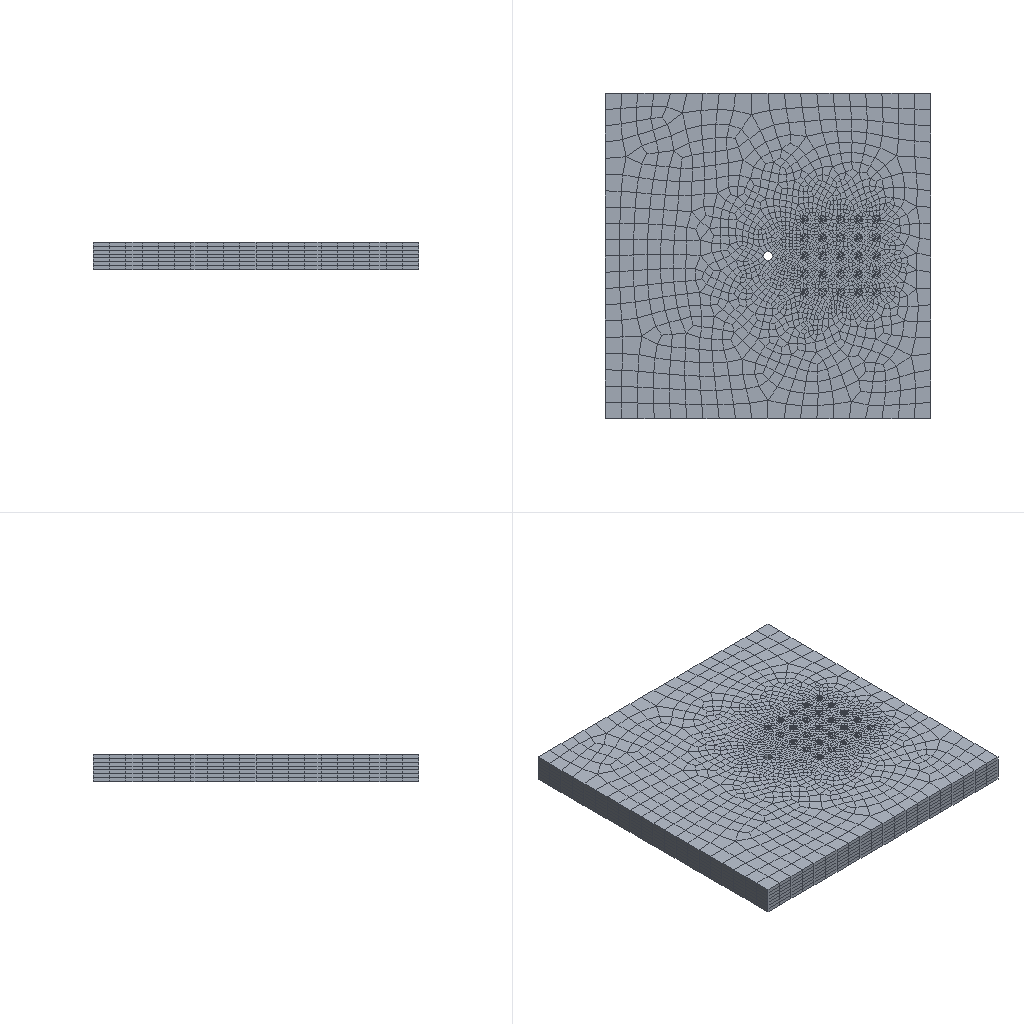Simulation study | abaqus
Set-up summary:
category,name,step,type,value,unit,region
solver,abaqus
solver,version,,,Abaqus/Standard 2020
units,not stated in the deck,,not stated
analysis,deck,,soils,soils
load_step,Step-1,Step-1,soils
load_step,requested,,,1
mesh,nodes,,,33552
mesh,elements,,,26299
element_type,C3D8R,,solid,13860
element_type,C3D8RP,,solid,12439
load,load commands in deck,,count,1
bc,support commands in deck,,count,5
material,SOIL,,in results
material,ZHUANG,,in results
check,setup vs results,,match,"per instance, exact: element labels, types and connectivity; labels of the nodes the elements use; coordinates of those nodes at SINGLE_PRECISION in 1 of 2 instance(s)"
Abaqus input file, long lists of numbers shortened:
*Heading
** Job name: Job-3 Model name: Model-1-Copy
** Generated by: Abaqus/CAE 2020
*Preprint, echo=NO, model=NO, history=NO, contact=NO
**
** PARTS
**
*Part, name=Part-1
*Node
      1,   17.1,           0.,           0.
      2,   15.3,           0.,           0.
** (15166 more lines like these left out)
*Element, type=C3D8RP
    1,   289,   327,   307,   328,  2185,  2223,  2203,  2224
    2,   327,   326,   306,   307,  2223,  2222,  2202,  2203
** (12437 more lines like these left out)
*Nset, nset=Set-1, generate
     1,  15168,      1
*Elset, elset=Set-1, generate
     1,  12439,      1
** Section: soil
*Solid Section, elset=Set-1, material=soil
,
*End Part
**
*Part, name=zhuang
*Node
      1,           3.,        -0.25,           0.
      2,           3.,        -0.25,          1.5
** (18382 more lines like these left out)
*Element, type=C3D8R
  1, 7899,  855,  870, 7901,  801,    1,   65,  803
  2, 7910, 7900,  857,  856,  812,  802,   52,   51
** (13858 more lines like these left out)
*Nset, nset=Set-1, generate
     1,  18384,      1
*Elset, elset=Set-1, generate
     1,  13860,      1
** Section: zhuang
*Solid Section, elset=Set-1, material=zhuang
,
*End Part
**
**
** ASSEMBLY
**
*Assembly, name=Assembly
**
*Instance, name=Part-1-1, part=Part-1
*End Instance
**
*Instance, name=zhuang-1, part=zhuang
          9.,          -9.,           0.
*End Instance
**
*Nset, nset=Set-1, instance=Part-1-1
     1,     2,     3,     4,     5,     6,     7,     8,     9,    10,    11,    12,    13,    14,    15,    16
    17,    33,    34,    35,    36,    37,    38,    39,    40,    41,    42,    43,    44,    45,    46,    47
** (19 more lines like these left out)
*Elset, elset=Set-1, instance=Part-1-1
    41,    42,    43,    44,    45,    46,    47,    48,    49,    50,    51,    52,    53,    54,    55,    56
    66,    67,    68,    97,    98,    99,   101,   102,   104,   105,   129,   181,   182,   195,   196,   232
** (16 more lines like these left out)
*Nset, nset=Set-2, instance=Part-1-1
    16,    17,    18,    19,    20,    21,    22,    23,    24,    25,    26,    27,    28,    29,    30,    31
    32,    33,    49,    50,    51,    52,    53,    54,    55,    56,    57,    58,    59,    60,    61,    62
** (19 more lines like these left out)
*Elset, elset=Set-2, instance=Part-1-1
    19,    20,    21,    56,    57,    75,    76,    77,    78,    91,    92,    93,    94,   100,   103,   104
   149,   150,   151,   158,   159,   160,   161,   182,   183,   197,   207,   215,   225,   226,   227,   228
** (16 more lines like these left out)
*Nset, nset=Set-3, instance=Part-1-1, generate
 13273,  15168,      1
*Nset, nset=Set-3, instance=zhuang-1
    2,    4,    6,    8,   10,   12,   14,   16,   18,   20,   22,   24,   26,   28,   30,   32
   34,   36,   38,   40,   42,   44,   46,   48,   50,   66,   67,   68,   69,   70,   71,   72
** (70 more lines like these left out)
*Elset, elset=Set-3, instance=Part-1-1, generate
 10663,  12439,      1
*Elset, elset=Set-3, instance=zhuang-1
   477,   478,   479,   480,   481,   482,   483,   484,   485,   486,   487,   488,   489,   490,   491,   492
   493,   494,   495,   496,   497,   498,   499,   500,   501,   502,   503,   504,   505,   506,   507,   508
** (56 more lines like these left out)
*Nset, nset=Set-4, instance=Part-1-1, generate
    1,  1896,     1
*Elset, elset=Set-4, instance=Part-1-1, generate
    1,  1777,     1
*Nset, nset=Set-5, instance=Part-1-1, generate
     1,  15168,      1
*Nset, nset=Set-5, instance=zhuang-1, generate
     1,  18384,      1
*Elset, elset=Set-5, instance=Part-1-1, generate
     1,  12439,      1
*Elset, elset=Set-5, instance=zhuang-1, generate
     1,  13860,      1
*Nset, nset=Set-6, instance=Part-1-1, generate
     1,  15168,      1
*Elset, elset=Set-6, instance=Part-1-1, generate
     1,  12439,      1
*Nset, nset=Set-7, instance=Part-1-1, generate
 13273,  15168,      1
*Elset, elset=Set-7, instance=Part-1-1, generate
 10663,  12439,      1
*Nset, nset=Set-8, instance=Part-1-1
    65,    66,    67,    68,    69,    70,    71,    72,  1961,  1962,  1963,  1964,  1965,  1966,  1967,  1968
  3857,  3858,  3859,  3860,  3861,  3862,  3863,  3864,  5753,  5754,  5755,  5756,  5757,  5758,  5759,  5760
** (2 more lines like these left out)
*Elset, elset=Set-8, instance=Part-1-1
   114,   116,   119,   234,   236,   798,   833,   834,  1891,  1893,  1896,  2011,  2013,  2575,  2610,  2611
  3668,  3670,  3673,  3788,  3790,  4352,  4387,  4388,  5445,  5447,  5450,  5565,  5567,  6129,  6164,  6165
** (2 more lines like these left out)
*Nset, nset=Set-9, instance=Part-1-1
    65,    66,    67,    68,    69,    70,    71,    72,  1961,  1962,  1963,  1964,  1965,  1966,  1967,  1968
  3857,  3858,  3859,  3860,  3861,  3862,  3863,  3864,  5753,  5754,  5755,  5756,  5757,  5758,  5759,  5760
** (2 more lines like these left out)
*Elset, elset=Set-9, instance=Part-1-1
   114,   116,   119,   234,   236,   798,   833,   834,  1891,  1893,  1896,  2011,  2013,  2575,  2610,  2611
  3668,  3670,  3673,  3788,  3790,  4352,  4387,  4388,  5445,  5447,  5450,  5565,  5567,  6129,  6164,  6165
** (2 more lines like these left out)
*Nset, nset=Set-10, instance=Part-1-1, generate
 13273,  15168,      1
*Nset, nset=Set-10, instance=zhuang-1
    2,    4,    6,    8,   10,   12,   14,   16,   18,   20,   22,   24,   26,   28,   30,   32
   34,   36,   38,   40,   42,   44,   46,   48,   50,   66,   67,   68,   69,   70,   71,   72
** (70 more lines like these left out)
*Elset, elset=Set-10, instance=Part-1-1, generate
 10663,  12439,      1
*Elset, elset=Set-10, instance=zhuang-1
   477,   478,   479,   480,   481,   482,   483,   484,   485,   486,   487,   488,   489,   490,   491,   492
   493,   494,   495,   496,   497,   498,   499,   500,   501,   502,   503,   504,   505,   506,   507,   508
** (56 more lines like these left out)
*Nset, nset=Set-11, instance=Part-1-1
 13273, 13274, 13275, 13276, 13277, 13278, 13279, 13280, 13281, 13282, 13283, 13284, 13285, 13286, 13287, 13288
 13289, 13290, 13291, 13292, 13293, 13294, 13295, 13296, 13297, 13298, 13299, 13300, 13301, 13302, 13303, 13304
** (116 more lines like these left out)
*Nset, nset=Set-11, instance=zhuang-1
    2,    4,    6,    8,   10,   12,   14,   16,   18,   20,   22,   24,   26,   28,   30,   32
   34,   36,   38,   40,   42,   44,   46,   48,   50,   66,   67,   68,   69,   70,   71,   72
** (70 more lines like these left out)
*Elset, elset=Set-11, instance=Part-1-1, generate
 10663,  12439,      1
*Elset, elset=Set-11, instance=zhuang-1
   477,   478,   479,   480,   481,   482,   483,   484,   485,   486,   487,   488,   489,   490,   491,   492
   493,   494,   495,   496,   497,   498,   499,   500,   501,   502,   503,   504,   505,   506,   507,   508
** (56 more lines like these left out)
*Nset, nset=Set-12, instance=Part-1-1
    1,    2,    3,    4,    5,    6,    7,    8,    9,   10,   11,   12,   13,   14,   15,   16
   17,   18,   19,   20,   21,   22,   23,   24,   25,   26,   27,   28,   29,   30,   31,   32
** (116 more lines like these left out)
*Elset, elset=Set-12, instance=Part-1-1, generate
    1,  1777,     1
*Elset, elset=_m_Surf-1_S4, internal, instance=Part-1-1
    31,    34,    36,    63,    64,    80,    84,   255,   257,   258,   262,   266,   277,   285,   297,   305
   308,   311,   330,   337,   356,   378,   379,   382,   389,   401,   406,   407,   421,   422,   432,   434
** (36 more lines like these left out)
*Elset, elset=_m_Surf-1_S3, internal, instance=Part-1-1
    27,    87,    88,   244,   259,   268,   274,   276,   286,   299,   301,   317,   319,   342,   355,   364
   373,   398,   413,   418,   442,   461,   850,   859,   862,   888,   890,   892,   897,   899,   907,   920
** (15 more lines like these left out)
*Elset, elset=_m_Surf-1_S5, internal, instance=Part-1-1
    29,    33,    65,    86,   248,   275,   298,   306,   310,   316,   324,   328,   329,   345,   369,   387
   414,   420,   427,   642,   649,   700,   802,   805,   806,   813,   816,   841,   844,   860,   868,   878
** (20 more lines like these left out)
*Elset, elset=_m_Surf-1_S6, internal, instance=Part-1-1
    62,    85,   243,   250,   261,   281,   283,   295,   302,   307,   314,   321,   322,   327,   352,   362
   367,   377,   429,   430,   463,   852,   874,   877,   896,   955,  1839,  1862,  2020,  2027,  2038,  2058
** (10 more lines like these left out)
*Surface, type=ELEMENT, name=m_Surf-1
_m_Surf-1_S4, S4
_m_Surf-1_S3, S3
_m_Surf-1_S6, S6
_m_Surf-1_S5, S5
*Elset, elset=_s_Surf-1_S4, internal, instance=zhuang-1
     1,    11,    12,    16,    35,    45,    46,    50,    69,    79,    80,    84,   103,   113,   114,   118
   137,   147,   148,   152,   171,   181,   182,   186,   205,   215,   216,   220,   239,   249,   250,   254
** (107 more lines like these left out)
*Elset, elset=_s_Surf-1_S5, internal, instance=zhuang-1
     2,    28,    36,    62,    70,    96,   104,   130,   138,   164,   172,   198,   206,   232,   240,   266
   274,   300,   308,   334,   342,   368,   376,   402,   410,   436,   444,   470,   478,   504,   512,   533
** (55 more lines like these left out)
*Elset, elset=_s_Surf-1_S3, internal, instance=zhuang-1
     4,    13,    14,    27,    31,    38,    47,    48,    61,    65,    72,    81,    82,    95,    99,   106
   115,   116,   129,   133,   140,   149,   150,   163,   167,   174,   183,   184,   197,   201,   208,   217
** (108 more lines like these left out)
*Elset, elset=_s_Surf-1_S6, internal, instance=zhuang-1
     5,     8,    17,    29,    32,    39,    42,    51,    63,    66,    73,    76,    85,    97,   100,   107
   110,   119,   131,   134,   141,   144,   153,   165,   168,   175,   178,   187,   199,   202,   209,   212
** (99 more lines like these left out)
*Surface, type=ELEMENT, name=s_Surf-1
_s_Surf-1_S4, S4
_s_Surf-1_S5, S5
_s_Surf-1_S6, S6
_s_Surf-1_S3, S3
** Constraint: Constraint-1
*Tie, name=Constraint-1, adjust=yes
s_Surf-1, m_Surf-1
*Nset, nset=Set-9_PP_, internal, instance=Part-1-1
    65,    66,    67,    68,    69,    70,    71,    72,  1961,  1962,  1963,  1964,  1965,  1966,  1967,  1968
  3857,  3858,  3859,  3860,  3861,  3862,  3863,  3864,  5753,  5754,  5755,  5756,  5757,  5758,  5759,  5760
** (2 more lines like these left out)
*Nset, nset=Set-12_PP_, internal, instance=Part-1-1
    1,    2,    3,    4,    5,    6,    7,    8,    9,   10,   11,   12,   13,   14,   15,   16
   17,   18,   19,   20,   21,   22,   23,   24,   25,   26,   27,   28,   29,   30,   31,   32
** (116 more lines like these left out)
*End Assembly
**
** MATERIALS
**
*Material, name=soil
*Density
1800.,
*Elastic
 1e+08, 0.3
*Gap Flow
 0.001,
*Permeability, specific=9800.
 6e-07, 0.48
*Mohr Coulomb
30., 0.01
*Mohr Coulomb Hardening
13000.,0.
*Material, name=zhuang
*Density
2000.,
*Elastic
 2e+10, 0.15
**
** INTERACTION PROPERTIES
**
*Surface Interaction, name=IntProp-1
1.,
*Friction, slip tolerance=0.005
 0.466,
*Surface Behavior, pressure-overclosure=HARD
**
** PREDEFINED FIELDS
**
** Name: Predefined Field-1   Type: Void ratio
*Initial Conditions, TYPE=RATIO
Set-5, 0.1
** ----------------------------------------------------------------
**
** STEP: Step-1
**
*Step, name=Step-1, nlgeom=YES, inc=100000
*Soils, utol=1.0, cetol=5., stabilize=0.0002, allsdtol=0.05, continue=NO
0.1, 1000., 0.01, 1000.,
**
** BOUNDARY CONDITIONS
**
** Name: BC-1 Type: 位移/转角
*Boundary
Set-1, 2, 2
** Name: BC-2 Type: 位移/转角
*Boundary
Set-2, 1, 1
** Name: BC-3 Type: 位移/转角
*Boundary
Set-11, 3, 3
** Name: BC-5 Type: 孔隙压力
*Boundary
Set-9_PP_, 8, 8, 30000.
** Name: [REDACTED] : Pore pressure
*Boundary
Set-12_PP_, 8, 8
**
** OUTPUT REQUESTS
**
*Restart, write, frequency=0
**
** FIELD OUTPUT: F-Output-1
**
*Output, field
*Node Output
CF, CFF, POR, RF, RM, RT, RVF, RVT
TF, U, V
*Element Output, directions=YES
ALEAKVRBXFEM, ALEAKVRTXFEM, CRDCUTXFEM, E, FLUVR, FLVEL, GELVR, GFVRXFEM, LE, LEAKVRBXFEM, LEAKVRTXFEM, MISES, MISESMAX, MISESONLY, PE, PEEQ
PEEQMAX, PEEQT, PFOPENXFEM, PFOPENXFEMCOMP, RD, S, SAT, SF, SSAVG, VEEQ, VOIDR, VVF, VVFG, VVFN, YIELDPOT
*Contact Output
CDISP, CSTRESS, PFL, PFLA, PTL, PTLA
**
** HISTORY OUTPUT: H-Output-1
**
*Output, history, variable=PRESELECT
*End Step
Results summary:
result,step,,partial,increments=40 time=970.811/1000.0
result,analysis,,,soils
result,last_loadstep,,,1
result,primary field,,,"U, POR"
result,reaction total,,FX,-1e-06,model units
result,reaction total,,FY,0.0,model units
result,reaction total,,FZ,2e-06,model units